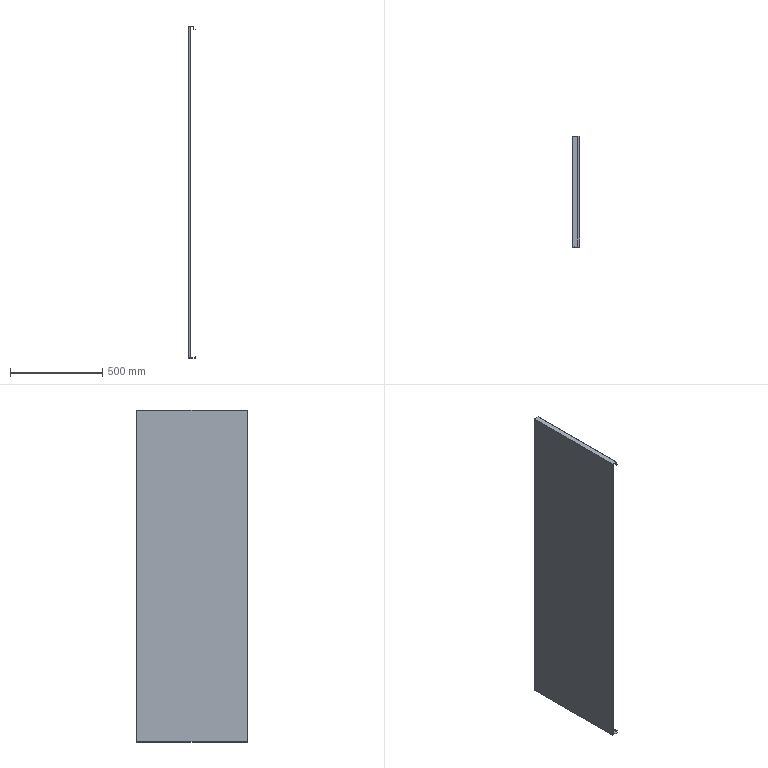Part | STEP file | 1 solid | 64 faces | box 40 x 600 x 1800 mm | volume 1173375 mm3 | plane 48 | cylinder 14 | spline 2 | commonest cylinder face diameters 0.4 x7 2.4 x7